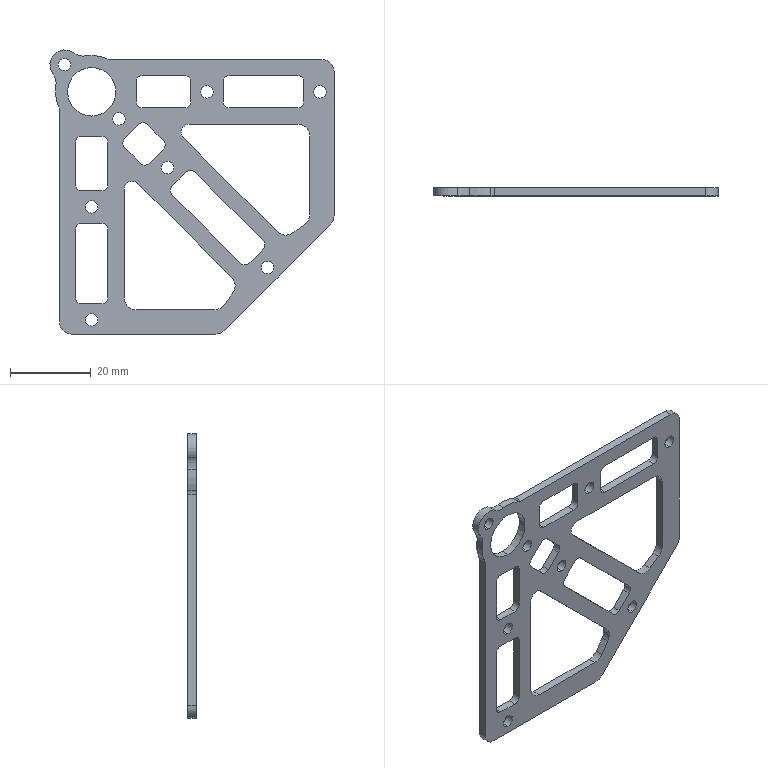Part | SolidWorks | features Fillet 4, Extrusion 1 | 1 solid | 103 faces | box 70.368 x 2 x 70.368 mm | volume 4319 mm3 | cylinder 64 | plane 39 | commonest cylinder face diameters 3 x26 3.1 x16 6 x10 4 x5 8 x2 12 x2